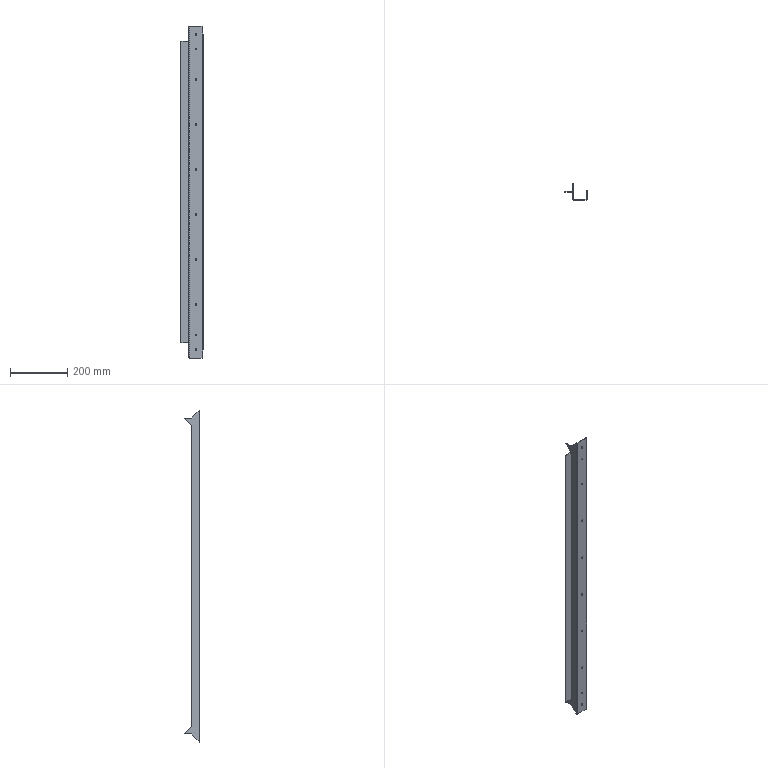Part | STEP file | SX-004-08 | 1 solid | 68 faces | box 78 x 55 x 1157 mm | volume 296255 mm3 | cylinder 34 | plane 32 | spline 2 | commonest cylinder face diameters 6 x16 8 x6 3 x4 0.4 x3 4.4 x3 4 x2